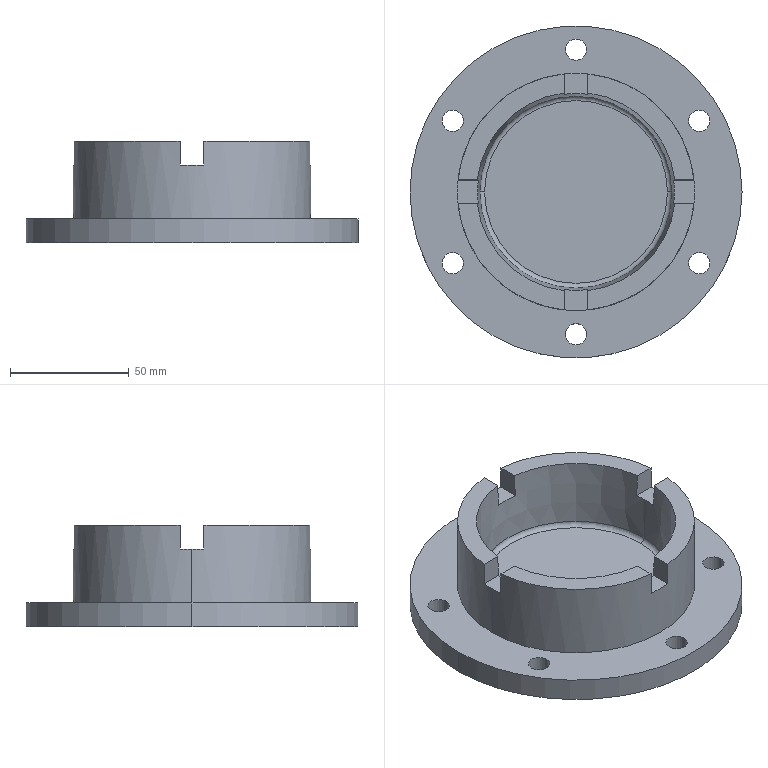Part | SolidWorks | features ICE 5, CirPattern 2, Fillet 1, Revolution 1 | 1 solid | 999 faces | box 140 x 140 x 42.75 mm | volume 226052 mm3 | plane 726 | spline 251 | cylinder 16 | torus 4 | cone 2 | commonest cylinder face diameters 9 x12 100 x2 140 x2